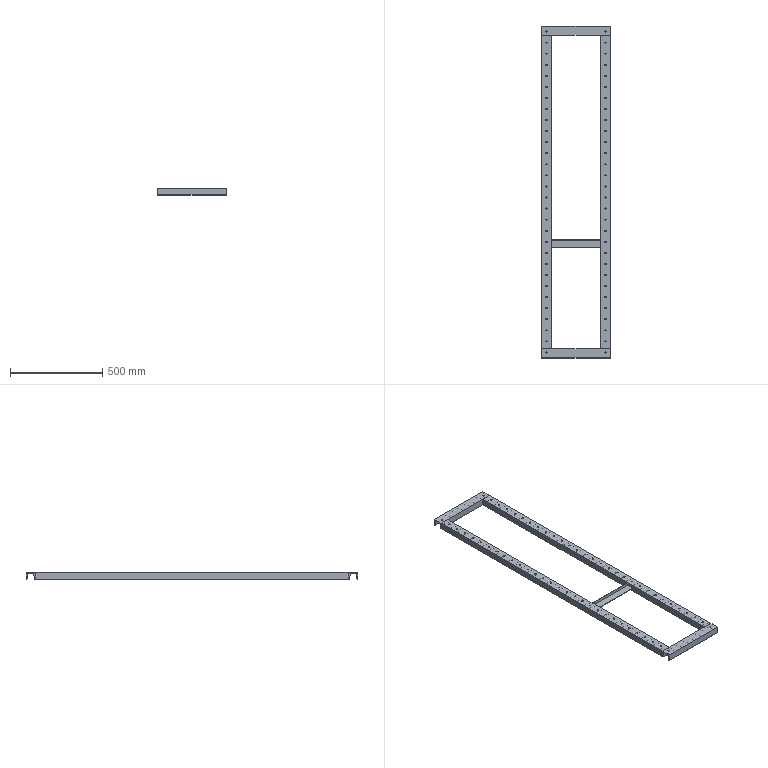Part | SolidWorks | features ICE 3, WeldMemberFeat 1, WeldmentFeature 1 | 5 solids | 184 faces | box 370 x 1800 x 37 mm | volume 2843417 mm3 | cylinder 136 | plane 48 | commonest cylinder face diameters 6.5 x120 7 x8 14 x8